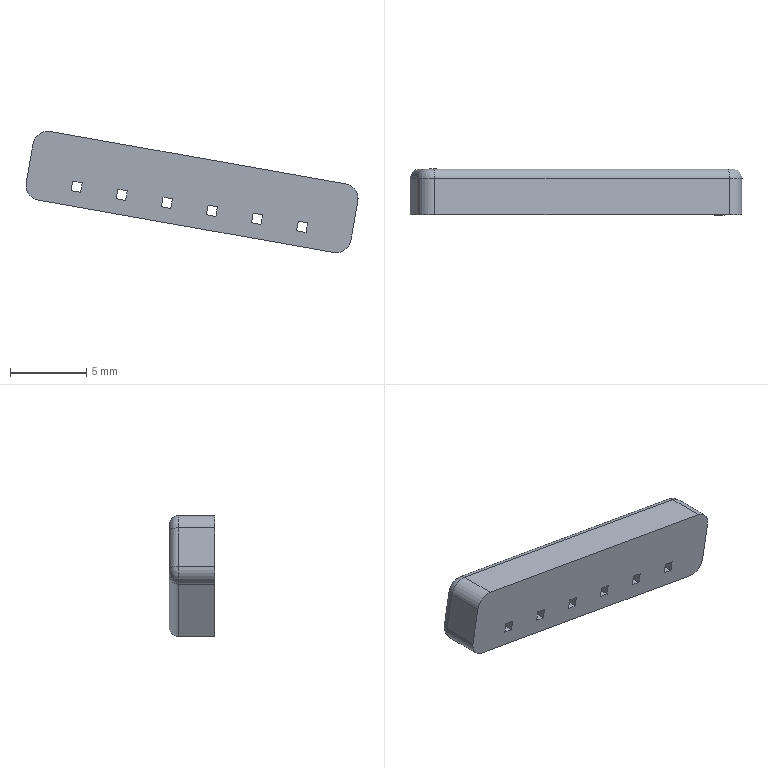Part | SolidWorks | features BaseBody 1 | 1 solid | 66 faces | box 21.746 x 3 x 7.946 mm | volume 278.91 mm3 | plane 54 | cylinder 8 | torus 4 | commonest cylinder face diameters 1.2 x4 2 x4